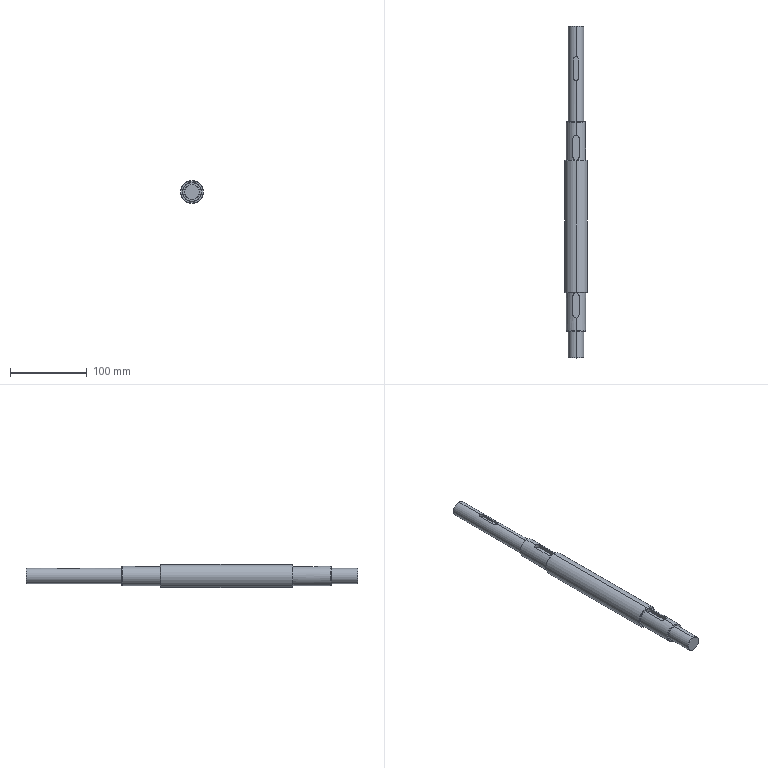Part | STEP file | LIELUN30_1-2 | 1 solid | 43 faces | box 30 x 432.6 x 30 mm | volume 218301 mm3 | cylinder 16 | plane 15 | cone 12 | commonest cylinder face diameters 8 x4 20 x4 25 x4 6 x2 30 x2
STEP:
#1=CARTESIAN_POINT('',(0.,85.5,15.));
#2=VERTEX_POINT('',#1);
#3=CARTESIAN_POINT('',(0.,85.5,-15.));
#4=VERTEX_POINT('',#3);
#5=CARTESIAN_POINT('',(0.,85.5,0.));
#6=DIRECTION('',(0.,1.,0.));
#7=DIRECTION('',(0.,0.,1.));
#8=AXIS2_PLACEMENT_3D('',#5,#6,#7);
#9=CIRCLE('',#8,15.);
#10=EDGE_CURVE('',#2,#4,#9,.T.);
#11=ORIENTED_EDGE('',*,*,#10,.T.);
#12=CARTESIAN_POINT('',(0.,257.1,-15.));
#13=VERTEX_POINT('',#12);
#14=CARTESIAN_POINT('',(0.,0.,-15.));
#15=DIRECTION('',(0.,1.,0.));
#16=VECTOR('',#15,1000.);
#17=LINE('',#14,#16);
#18=EDGE_CURVE('',#4,#13,#17,.T.);
#19=ORIENTED_EDGE('',*,*,#18,.T.);
#20=CARTESIAN_POINT('',(0.,257.1,15.));
#21=VERTEX_POINT('',#20);
#22=CARTESIAN_POINT('',(0.,257.1,0.));
#23=DIRECTION('',(0.,-1.,0.));
#24=DIRECTION('',(0.,0.,1.));
#25=AXIS2_PLACEMENT_3D('',#22,#23,#24);
#26=CIRCLE('',#25,15.);
#27=EDGE_CURVE('',#13,#21,#26,.T.);
#28=ORIENTED_EDGE('',*,*,#27,.T.);
#29=CARTESIAN_POINT('',(0.,0.,15.));
#30=DIRECTION('',(0.,1.,0.));
#31=VECTOR('',#30,1000.);
#32=LINE('',#29,#31);
#33=EDGE_CURVE('',#2,#21,#32,.T.);
#34=ORIENTED_EDGE('',*,*,#33,.F.);
#35=EDGE_LOOP('',(#11,#19,#28,#34));
#36=FACE_OUTER_BOUND('',#35,.T.);
#37=CARTESIAN_POINT('',(0.,0.,0.));
#38=DIRECTION('',(0.,1.,0.));
#39=DIRECTION('',(0.,0.,1.));
#40=AXIS2_PLACEMENT_3D('',#37,#38,#39);
#41=CYLINDRICAL_SURFACE('',#40,15.);
#42=ADVANCED_FACE('',(#36),#41,.T.);
#43=CARTESIAN_POINT('',(0.,257.6,-14.5));
#44=VERTEX_POINT('',#43);
#45=CARTESIAN_POINT('',(0.,257.6,14.5));
#46=VERTEX_POINT('',#45);
#47=CARTESIAN_POINT('',(0.,257.6,0.));
#48=DIRECTION('',(0.,-1.,0.));
#49=DIRECTION('',(0.,0.,-1.));
#50=AXIS2_PLACEMENT_3D('',#47,#48,#49);
#51=CIRCLE('',#50,14.5);
#52=EDGE_CURVE('',#44,#46,#51,.T.);
#53=ORIENTED_EDGE('',*,*,#52,.T.);
#54=CARTESIAN_POINT('',(0.,257.1,15.));
#55=DIRECTION('',(0.,-0.7071,0.7071));
#56=VECTOR('',#55,1000.);
#57=LINE('',#54,#56);
#58=EDGE_CURVE('',#46,#21,#57,.T.);
#59=ORIENTED_EDGE('',*,*,#58,.T.);
#60=ORIENTED_EDGE('',*,*,#27,.F.);
#61=CARTESIAN_POINT('',(0.,257.1,-15.));
#62=DIRECTION('',(0.,-0.7071,-0.7071));
#63=VECTOR('',#62,1000.);
#64=LINE('',#61,#63);
#65=EDGE_CURVE('',#44,#13,#64,.T.);
#66=ORIENTED_EDGE('',*,*,#65,.F.);
#67=EDGE_LOOP('',(#53,#59,#60,#66));
#68=FACE_OUTER_BOUND('',#67,.T.);
#69=CARTESIAN_POINT('',(0.,257.1,0.));
#70=DIRECTION('',(0.,-1.,0.));
#71=DIRECTION('',(0.,0.,-1.));
#72=AXIS2_PLACEMENT_3D('',#69,#70,#71);
#73=CONICAL_SURFACE('',#72,15.,0.7854);
#74=ADVANCED_FACE('',(#68),#73,.T.);
#75=CARTESIAN_POINT('',(0.,85.,14.5));
#76=VERTEX_POINT('',#75);
#77=CARTESIAN_POINT('',(0.,85.,-14.5));
#78=VERTEX_POINT('',#77);
#79=CARTESIAN_POINT('',(0.,85.,0.));
#80=DIRECTION('',(0.,1.,0.));
#81=DIRECTION('',(0.,0.,1.));
#82=AXIS2_PLACEMENT_3D('',#79,#80,#81);
#83=CIRCLE('',#82,14.5);
#84=EDGE_CURVE('',#76,#78,#83,.T.);
#85=ORIENTED_EDGE('',*,*,#84,.T.);
#86=CARTESIAN_POINT('',(0.,85.5,-15.));
#87=DIRECTION('',(0.,0.7071,-0.7071));
#88=VECTOR('',#87,1000.);
#89=LINE('',#86,#88);
#90=EDGE_CURVE('',#78,#4,#89,.T.);
#91=ORIENTED_EDGE('',*,*,#90,.T.);
#92=ORIENTED_EDGE('',*,*,#10,.F.);
#93=CARTESIAN_POINT('',(0.,85.5,15.));
#94=DIRECTION('',(0.,0.7071,0.7071));
#95=VECTOR('',#94,1000.);
#96=LINE('',#93,#95);
#97=EDGE_CURVE('',#76,#2,#96,.T.);
#98=ORIENTED_EDGE('',*,*,#97,.F.);
#99=EDGE_LOOP('',(#85,#91,#92,#98));
#100=FACE_OUTER_BOUND('',#99,.T.);
#101=CARTESIAN_POINT('',(0.,85.5,0.));
#102=DIRECTION('',(0.,1.,0.));
#103=DIRECTION('',(0.,0.,1.));
#104=AXIS2_PLACEMENT_3D('',#101,#102,#103);
#105=CONICAL_SURFACE('',#104,15.,0.7854);
#106=ADVANCED_FACE('',(#100),#105,.T.);
#107=CARTESIAN_POINT('',(0.,257.6,-12.5));
#108=VERTEX_POINT('',#107);
#109=CARTESIAN_POINT('',(0.,257.6,12.5));
#110=VERTEX_POINT('',#109);
#111=CARTESIAN_POINT('',(0.,257.6,0.));
#112=DIRECTION('',(0.,-1.,0.));
#113=DIRECTION('',(0.,0.,1.));
#114=AXIS2_PLACEMENT_3D('',#111,#112,#113);
#115=CIRCLE('',#114,12.5);
#116=EDGE_CURVE('',#108,#110,#115,.T.);
#117=ORIENTED_EDGE('',*,*,#116,.F.);
#118=CARTESIAN_POINT('',(0.,307.1,-12.5));
#119=VERTEX_POINT('',#118);
#120=CARTESIAN_POINT('',(0.,432.6,-12.5));
#121=DIRECTION('',(0.,1.,0.));
#122=VECTOR('',#121,1000.);
#123=LINE('',#120,#122);
#124=EDGE_CURVE('',#108,#119,#123,.T.);
#125=ORIENTED_EDGE('',*,*,#124,.T.);
#126=CARTESIAN_POINT('',(0.,307.1,12.5));
#127=VERTEX_POINT('',#126);
#128=CARTESIAN_POINT('',(0.,307.1,0.));
#129=DIRECTION('',(0.,-1.,0.));
#130=DIRECTION('',(0.,0.,1.));
#131=AXIS2_PLACEMENT_3D('',#128,#129,#130);
#132=CIRCLE('',#131,12.5);
#133=EDGE_CURVE('',#119,#127,#132,.T.);
#134=ORIENTED_EDGE('',*,*,#133,.T.);
#135=CARTESIAN_POINT('',(0.,290.6,12.5));
#136=VERTEX_POINT('',#135);
#137=CARTESIAN_POINT('',(0.,432.6,12.5));
#138=DIRECTION('',(0.,1.,0.));
#139=VECTOR('',#138,1000.);
#140=LINE('',#137,#139);
#141=EDGE_CURVE('',#136,#127,#140,.T.);
#142=ORIENTED_EDGE('',*,*,#141,.F.);
#143=CARTESIAN_POINT('',(4.,286.6,11.843));
#144=VERTEX_POINT('',#143);
#145=CARTESIAN_POINT('',(0.,290.6,12.5));
#146=CARTESIAN_POINT('',(0.266,290.6,12.5));
#147=CARTESIAN_POINT('',(0.5272,290.574,12.492));
#148=CARTESIAN_POINT('',(1.041,290.471,12.459));
#149=CARTESIAN_POINT('',(1.296,290.393,12.435));
#150=CARTESIAN_POINT('',(1.779,290.192,12.375));
#151=CARTESIAN_POINT('',(2.008,290.069,12.34));
#152=CARTESIAN_POINT('',(2.441,289.779,12.261));
#153=CARTESIAN_POINT('',(2.645,289.612,12.218));
#154=CARTESIAN_POINT('',(3.011,289.246,12.133));
#155=CARTESIAN_POINT('',(3.176,289.046,12.091));
#156=CARTESIAN_POINT('',(3.469,288.609,12.01));
#157=CARTESIAN_POINT('',(3.592,288.38,11.973));
#158=CARTESIAN_POINT('',(3.792,287.9,11.911));
#159=CARTESIAN_POINT('',(3.87,287.646,11.886));
#160=CARTESIAN_POINT('',(3.974,287.128,11.852));
#161=CARTESIAN_POINT('',(4.,286.866,11.843));
#162=CARTESIAN_POINT('',(4.,286.6,11.843));
#163=B_SPLINE_CURVE_WITH_KNOTS('',3,(#145,#146,#147,#148,#149,#150,#151,#152,#153,#154,#155,#156,#157,#158,#159,#160,#161,#162),.UNSPECIFIED.,.F.,.F.,(4,2,2,2,2,2,2,2,4),(0.00629,0.007077,0.007863,0.008649,0.009436,0.01022,0.01101,0.01179,0.01258),.UNSPECIFIED.);
#164=EDGE_CURVE('',#136,#144,#163,.T.);
#165=ORIENTED_EDGE('',*,*,#164,.T.);
#166=CARTESIAN_POINT('',(4.,261.6,11.843));
#167=VERTEX_POINT('',#166);
#168=CARTESIAN_POINT('',(4.,432.6,11.843));
#169=DIRECTION('',(0.,-1.,0.));
#170=VECTOR('',#169,1000.);
#171=LINE('',#168,#170);
#172=EDGE_CURVE('',#144,#167,#171,.T.);
#173=ORIENTED_EDGE('',*,*,#172,.T.);
#174=CARTESIAN_POINT('',(4.,261.6,11.843));
#175=CARTESIAN_POINT('',(4.,261.334,11.843));
#176=CARTESIAN_POINT('',(3.974,261.073,11.852));
#177=CARTESIAN_POINT('',(3.871,260.56,11.886));
#178=CARTESIAN_POINT('',(3.794,260.305,11.911));
#179=CARTESIAN_POINT('',(3.592,259.821,11.973));
#180=CARTESIAN_POINT('',(3.47,259.593,12.01));
#181=CARTESIAN_POINT('',(3.18,259.159,12.09));
#182=CARTESIAN_POINT('',(3.012,258.956,12.133));
#183=CARTESIAN_POINT('',(2.646,258.589,12.218));
#184=CARTESIAN_POINT('',(2.446,258.424,12.26));
#185=CARTESIAN_POINT('',(2.01,258.132,12.339));
#186=CARTESIAN_POINT('',(1.78,258.009,12.375));
#187=CARTESIAN_POINT('',(1.3,257.808,12.435));
#188=CARTESIAN_POINT('',(1.047,257.73,12.459));
#189=CARTESIAN_POINT('',(0.5285,257.626,12.492));
#190=CARTESIAN_POINT('',(0.266,257.6,12.5));
#191=CARTESIAN_POINT('',(0.,257.6,12.5));
#192=B_SPLINE_CURVE_WITH_KNOTS('',3,(#174,#175,#176,#177,#178,#179,#180,#181,#182,#183,#184,#185,#186,#187,#188,#189,#190,#191),.UNSPECIFIED.,.F.,.F.,(4,2,2,2,2,2,2,2,4),(0.,0.0007863,0.001573,0.002359,0.003145,0.003931,0.004718,0.005504,0.00629),.UNSPECIFIED.);
#193=EDGE_CURVE('',#167,#110,#192,.T.);
#194=ORIENTED_EDGE('',*,*,#193,.T.);
#195=EDGE_LOOP('',(#117,#125,#134,#142,#165,#173,#194));
#196=FACE_OUTER_BOUND('',#195,.T.);
#197=CARTESIAN_POINT('',(0.,432.6,0.));
#198=DIRECTION('',(0.,1.,0.));
#199=DIRECTION('',(0.,0.,1.));
#200=AXIS2_PLACEMENT_3D('',#197,#198,#199);
#201=CYLINDRICAL_SURFACE('',#200,12.5);
#202=ADVANCED_FACE('',(#196),#201,.T.);
#203=CARTESIAN_POINT('',(4.,56.,11.843));
#204=VERTEX_POINT('',#203);
#205=CARTESIAN_POINT('',(0.,52.,12.5));
#206=VERTEX_POINT('',#205);
#207=CARTESIAN_POINT('',(4.,56.,11.843));
#208=CARTESIAN_POINT('',(4.,55.734,11.843));
#209=CARTESIAN_POINT('',(3.974,55.473,11.852));
#210=CARTESIAN_POINT('',(3.871,54.96,11.886));
#211=CARTESIAN_POINT('',(3.794,54.705,11.911));
#212=CARTESIAN_POINT('',(3.592,54.221,11.973));
#213=CARTESIAN_POINT('',(3.47,53.993,12.01));
#214=CARTESIAN_POINT('',(3.18,53.559,12.09));
#215=CARTESIAN_POINT('',(3.012,53.356,12.133));
#216=CARTESIAN_POINT('',(2.646,52.989,12.218));
#217=CARTESIAN_POINT('',(2.446,52.824,12.26));
#218=CARTESIAN_POINT('',(2.01,52.532,12.339));
#219=CARTESIAN_POINT('',(1.78,52.409,12.375));
#220=CARTESIAN_POINT('',(1.3,52.208,12.435));
#221=CARTESIAN_POINT('',(1.047,52.13,12.459));
#222=CARTESIAN_POINT('',(0.5285,52.026,12.492));
#223=CARTESIAN_POINT('',(0.266,52.,12.5));
#224=CARTESIAN_POINT('',(0.,52.,12.5));
#225=B_SPLINE_CURVE_WITH_KNOTS('',3,(#207,#208,#209,#210,#211,#212,#213,#214,#215,#216,#217,#218,#219,#220,#221,#222,#223,#224),.UNSPECIFIED.,.F.,.F.,(4,2,2,2,2,2,2,2,4),(-0.00629,-0.005504,-0.004718,-0.003932,-0.003145,-0.002359,-0.001573,-0.0007863,0.),.UNSPECIFIED.);
#226=EDGE_CURVE('',#204,#206,#225,.T.);
#227=ORIENTED_EDGE('',*,*,#226,.T.);
#228=CARTESIAN_POINT('',(0.,35.5,12.5));
#229=VERTEX_POINT('',#228);
#230=CARTESIAN_POINT('',(0.,0.,12.5));
#231=DIRECTION('',(0.,-1.,0.));
#232=VECTOR('',#231,1000.);
#233=LINE('',#230,#232);
#234=EDGE_CURVE('',#206,#229,#233,.T.);
#235=ORIENTED_EDGE('',*,*,#234,.T.);
#236=CARTESIAN_POINT('',(12.5,35.5,0.));
#237=VERTEX_POINT('',#236);
#238=CARTESIAN_POINT('',(0.,35.5,0.));
#239=DIRECTION('',(0.,1.,0.));
#240=DIRECTION('',(0.,0.,-1.));
#241=AXIS2_PLACEMENT_3D('',#238,#239,#240);
#242=CIRCLE('',#241,12.5);
#243=EDGE_CURVE('',#229,#237,#242,.T.);
#244=ORIENTED_EDGE('',*,*,#243,.T.);
#245=CARTESIAN_POINT('',(0.,35.5,-12.5));
#246=VERTEX_POINT('',#245);
#247=CARTESIAN_POINT('',(0.,35.5,0.));
#248=DIRECTION('',(0.,1.,0.));
#249=DIRECTION('',(0.,0.,-1.));
#250=AXIS2_PLACEMENT_3D('',#247,#248,#249);
#251=CIRCLE('',#250,12.5);
#252=EDGE_CURVE('',#237,#246,#251,.T.);
#253=ORIENTED_EDGE('',*,*,#252,.T.);
#254=CARTESIAN_POINT('',(0.,85.,-12.5));
#255=VERTEX_POINT('',#254);
#256=CARTESIAN_POINT('',(0.,0.,-12.5));
#257=DIRECTION('',(0.,-1.,0.));
#258=VECTOR('',#257,1000.);
#259=LINE('',#256,#258);
#260=EDGE_CURVE('',#255,#246,#259,.T.);
#261=ORIENTED_EDGE('',*,*,#260,.F.);
#262=CARTESIAN_POINT('',(0.,85.,12.5));
#263=VERTEX_POINT('',#262);
#264=CARTESIAN_POINT('',(0.,85.,0.));
#265=DIRECTION('',(0.,1.,0.));
#266=DIRECTION('',(0.,0.,-1.));
#267=AXIS2_PLACEMENT_3D('',#264,#265,#266);
#268=CIRCLE('',#267,12.5);
#269=EDGE_CURVE('',#263,#255,#268,.T.);
#270=ORIENTED_EDGE('',*,*,#269,.F.);
#271=CARTESIAN_POINT('',(4.,81.,11.843));
#272=VERTEX_POINT('',#271);
#273=CARTESIAN_POINT('',(0.,85.,12.5));
#274=CARTESIAN_POINT('',(0.266,85.,12.5));
#275=CARTESIAN_POINT('',(0.5272,84.974,12.492));
#276=CARTESIAN_POINT('',(1.041,84.871,12.459));
#277=CARTESIAN_POINT('',(1.296,84.793,12.435));
#278=CARTESIAN_POINT('',(1.779,84.592,12.375));
#279=CARTESIAN_POINT('',(2.008,84.469,12.34));
#280=CARTESIAN_POINT('',(2.441,84.179,12.261));
#281=CARTESIAN_POINT('',(2.645,84.012,12.218));
#282=CARTESIAN_POINT('',(3.011,83.646,12.133));
#283=CARTESIAN_POINT('',(3.176,83.446,12.091));
#284=CARTESIAN_POINT('',(3.469,83.009,12.01));
#285=CARTESIAN_POINT('',(3.592,82.78,11.973));
#286=CARTESIAN_POINT('',(3.792,82.3,11.911));
#287=CARTESIAN_POINT('',(3.87,82.046,11.886));
#288=CARTESIAN_POINT('',(3.974,81.528,11.852));
#289=CARTESIAN_POINT('',(4.,81.266,11.843));
#290=CARTESIAN_POINT('',(4.,81.,11.843));
#291=B_SPLINE_CURVE_WITH_KNOTS('',3,(#273,#274,#275,#276,#277,#278,#279,#280,#281,#282,#283,#284,#285,#286,#287,#288,#289,#290),.UNSPECIFIED.,.F.,.F.,(4,2,2,2,2,2,2,2,4),(0.,0.0007863,0.001573,0.002359,0.003145,0.003932,0.004718,0.005504,0.00629),.UNSPECIFIED.);
#292=EDGE_CURVE('',#263,#272,#291,.T.);
#293=ORIENTED_EDGE('',*,*,#292,.T.);
#294=CARTESIAN_POINT('',(4.,0.,11.843));
#295=DIRECTION('',(0.,-1.,0.));
#296=VECTOR('',#295,1000.);
#297=LINE('',#294,#296);
#298=EDGE_CURVE('',#272,#204,#297,.T.);
#299=ORIENTED_EDGE('',*,*,#298,.T.);
#300=EDGE_LOOP('',(#227,#235,#244,#253,#261,#270,#293,#299));
#301=FACE_OUTER_BOUND('',#300,.T.);
#302=CARTESIAN_POINT('',(0.,0.,0.));
#303=DIRECTION('',(0.,-1.,0.));
#304=DIRECTION('',(0.,0.,-1.));
#305=AXIS2_PLACEMENT_3D('',#302,#303,#304);
#306=CYLINDRICAL_SURFACE('',#305,12.5);
#307=ADVANCED_FACE('',(#301),#306,.T.);
#308=CARTESIAN_POINT('',(0.,307.6,-12.));
#309=VERTEX_POINT('',#308);
#310=CARTESIAN_POINT('',(0.,307.6,12.));
#311=VERTEX_POINT('',#310);
#312=CARTESIAN_POINT('',(0.,307.6,0.));
#313=DIRECTION('',(0.,-1.,0.));
#314=DIRECTION('',(0.,0.,-1.));
#315=AXIS2_PLACEMENT_3D('',#312,#313,#314);
#316=CIRCLE('',#315,12.);
#317=EDGE_CURVE('',#309,#311,#316,.T.);
#318=ORIENTED_EDGE('',*,*,#317,.T.);
#319=CARTESIAN_POINT('',(0.,307.1,12.5));
#320=DIRECTION('',(0.,-0.7071,0.7071));
#321=VECTOR('',#320,1000.);
#322=LINE('',#319,#321);
#323=EDGE_CURVE('',#311,#127,#322,.T.);
#324=ORIENTED_EDGE('',*,*,#323,.T.);
#325=ORIENTED_EDGE('',*,*,#133,.F.);
#326=CARTESIAN_POINT('',(0.,307.1,-12.5));
#327=DIRECTION('',(0.,-0.7071,-0.7071));
#328=VECTOR('',#327,1000.);
#329=LINE('',#326,#328);
#330=EDGE_CURVE('',#309,#119,#329,.T.);
#331=ORIENTED_EDGE('',*,*,#330,.F.);
#332=EDGE_LOOP('',(#318,#324,#325,#331));
#333=FACE_OUTER_BOUND('',#332,.T.);
#334=CARTESIAN_POINT('',(0.,307.1,0.));
#335=DIRECTION('',(0.,-1.,0.));
#336=DIRECTION('',(0.,0.,-1.));
#337=AXIS2_PLACEMENT_3D('',#334,#335,#336);
#338=CONICAL_SURFACE('',#337,12.5,0.7854);
#339=ADVANCED_FACE('',(#333),#338,.T.);
#340=CARTESIAN_POINT('',(-12.,35.,0.));
#341=VERTEX_POINT('',#340);
#342=CARTESIAN_POINT('',(12.,35.,0.));
#343=VERTEX_POINT('',#342);
#344=CARTESIAN_POINT('',(0.,35.,0.));
#345=DIRECTION('',(0.,1.,0.));
#346=DIRECTION('',(-1.,0.,0.));
#347=AXIS2_PLACEMENT_3D('',#344,#345,#346);
#348=CIRCLE('',#347,12.);
#349=EDGE_CURVE('',#341,#343,#348,.T.);
#350=ORIENTED_EDGE('',*,*,#349,.T.);
#351=CARTESIAN_POINT('',(12.5,35.5,0.));
#352=DIRECTION('',(0.7071,0.7071,0.));
#353=VECTOR('',#352,1000.);
#354=LINE('',#351,#353);
#355=EDGE_CURVE('',#343,#237,#354,.T.);
#356=ORIENTED_EDGE('',*,*,#355,.T.);
#357=ORIENTED_EDGE('',*,*,#243,.F.);
#358=CARTESIAN_POINT('',(-12.5,35.5,0.));
#359=VERTEX_POINT('',#358);
#360=CARTESIAN_POINT('',(0.,35.5,0.));
#361=DIRECTION('',(0.,1.,0.));
#362=DIRECTION('',(0.,0.,-1.));
#363=AXIS2_PLACEMENT_3D('',#360,#361,#362);
#364=CIRCLE('',#363,12.5);
#365=EDGE_CURVE('',#359,#229,#364,.T.);
#366=ORIENTED_EDGE('',*,*,#365,.F.);
#367=CARTESIAN_POINT('',(-12.5,35.5,0.));
#368=DIRECTION('',(-0.7071,0.7071,0.));
#369=VECTOR('',#368,1000.);
#370=LINE('',#367,#369);
#371=EDGE_CURVE('',#341,#359,#370,.T.);
#372=ORIENTED_EDGE('',*,*,#371,.F.);
#373=EDGE_LOOP('',(#350,#356,#357,#366,#372));
#374=FACE_OUTER_BOUND('',#373,.T.);
#375=CARTESIAN_POINT('',(0.,35.5,0.));
#376=DIRECTION('',(0.,1.,0.));
#377=DIRECTION('',(-1.,0.,0.));
#378=AXIS2_PLACEMENT_3D('',#375,#376,#377);
#379=CONICAL_SURFACE('',#378,12.5,0.7854);
#380=ADVANCED_FACE('',(#374),#379,.T.);
#381=CARTESIAN_POINT('',(0.,307.6,-10.));
#382=VERTEX_POINT('',#381);
#383=CARTESIAN_POINT('',(0.,307.6,10.));
#384=VERTEX_POINT('',#383);
#385=CARTESIAN_POINT('',(0.,307.6,0.));
#386=DIRECTION('',(0.,-1.,0.));
#387=DIRECTION('',(0.,0.,1.));
#388=AXIS2_PLACEMENT_3D('',#385,#386,#387);
#389=CIRCLE('',#388,10.);
#390=EDGE_CURVE('',#382,#384,#389,.T.);
#391=ORIENTED_EDGE('',*,*,#390,.F.);
#392=CARTESIAN_POINT('',(0.,432.1,-10.));
#393=VERTEX_POINT('',#392);
#394=CARTESIAN_POINT('',(0.,432.6,-10.));
#395=DIRECTION('',(0.,1.,0.));
#396=VECTOR('',#395,1000.);
#397=LINE('',#394,#396);
#398=EDGE_CURVE('',#382,#393,#397,.T.);
#399=ORIENTED_EDGE('',*,*,#398,.T.);
#400=CARTESIAN_POINT('',(0.,432.1,10.));
#401=VERTEX_POINT('',#400);
#402=CARTESIAN_POINT('',(0.,432.1,0.));
#403=DIRECTION('',(0.,-1.,0.));
#404=DIRECTION('',(0.,0.,1.));
#405=AXIS2_PLACEMENT_3D('',#402,#403,#404);
#406=CIRCLE('',#405,10.);
#407=EDGE_CURVE('',#393,#401,#406,.T.);
#408=ORIENTED_EDGE('',*,*,#407,.T.);
#409=CARTESIAN_POINT('',(0.,392.6,10.));
#410=VERTEX_POINT('',#409);
#411=CARTESIAN_POINT('',(0.,432.6,10.));
#412=DIRECTION('',(0.,1.,0.));
#413=VECTOR('',#412,1000.);
#414=LINE('',#411,#413);
#415=EDGE_CURVE('',#410,#401,#414,.T.);
#416=ORIENTED_EDGE('',*,*,#415,.F.);
#417=CARTESIAN_POINT('',(3.,389.6,9.539));
#418=VERTEX_POINT('',#417);
#419=CARTESIAN_POINT('',(0.,392.6,10.));
#420=CARTESIAN_POINT('',(0.1993,392.6,10.));
#421=CARTESIAN_POINT('',(0.3951,392.58,9.994));
#422=CARTESIAN_POINT('',(0.7799,392.503,9.971));
#423=CARTESIAN_POINT('',(0.971,392.445,9.954));
#424=CARTESIAN_POINT('',(1.334,392.294,9.912));
#425=CARTESIAN_POINT('',(1.505,392.202,9.887));
#426=CARTESIAN_POINT('',(1.831,391.985,9.832));
#427=CARTESIAN_POINT('',(1.984,391.859,9.802));
#428=CARTESIAN_POINT('',(2.396,391.447,9.713));
#429=CARTESIAN_POINT('',(2.619,391.114,9.652));
#430=CARTESIAN_POINT('',(2.844,390.574,9.587));
#431=CARTESIAN_POINT('',(2.902,390.384,9.57));
#432=CARTESIAN_POINT('',(2.98,389.996,9.546));
#433=CARTESIAN_POINT('',(3.,389.799,9.539));
#434=CARTESIAN_POINT('',(3.,389.6,9.539));
#435=B_SPLINE_CURVE_WITH_KNOTS('',3,(#419,#420,#421,#422,#423,#424,#425,#426,#427,#428,#429,#430,#431,#432,#433,#434),.UNSPECIFIED.,.F.,.F.,(4,2,2,2,2,2,2,4),(0.004714,0.005303,0.005892,0.006481,0.007071,0.008249,0.008838,0.009428),.UNSPECIFIED.);
#436=EDGE_CURVE('',#410,#418,#435,.T.);
#437=ORIENTED_EDGE('',*,*,#436,.T.);
#438=CARTESIAN_POINT('',(3.,364.6,9.539));
#439=VERTEX_POINT('',#438);
#440=CARTESIAN_POINT('',(3.,432.6,9.539));
#441=DIRECTION('',(0.,-1.,0.));
#442=VECTOR('',#441,1000.);
#443=LINE('',#440,#442);
#444=EDGE_CURVE('',#418,#439,#443,.T.);
#445=ORIENTED_EDGE('',*,*,#444,.T.);
#446=CARTESIAN_POINT('',(0.,361.6,10.));
#447=VERTEX_POINT('',#446);
#448=CARTESIAN_POINT('',(3.,364.6,9.539));
#449=CARTESIAN_POINT('',(3.,364.401,9.539));
#450=CARTESIAN_POINT('',(2.98,364.205,9.546));
#451=CARTESIAN_POINT('',(2.904,363.82,9.569));
#452=CARTESIAN_POINT('',(2.845,363.629,9.587));
#453=CARTESIAN_POINT('',(2.695,363.267,9.63));
#454=CARTESIAN_POINT('',(2.602,363.095,9.656));
#455=CARTESIAN_POINT('',(2.385,362.77,9.712));
#456=CARTESIAN_POINT('',(2.259,362.617,9.742));
#457=CARTESIAN_POINT('',(1.847,362.204,9.832));
#458=CARTESIAN_POINT('',(1.515,361.981,9.891));
#459=CARTESIAN_POINT('',(0.9743,361.756,9.954));
#460=CARTESIAN_POINT('',(0.7845,361.698,9.971));
#461=CARTESIAN_POINT('',(0.3961,361.62,9.994));
#462=CARTESIAN_POINT('',(0.1993,361.6,10.));
#463=CARTESIAN_POINT('',(0.,361.6,10.));
#464=B_SPLINE_CURVE_WITH_KNOTS('',3,(#448,#449,#450,#451,#452,#453,#454,#455,#456,#457,#458,#459,#460,#461,#462,#463),.UNSPECIFIED.,.F.,.F.,(4,2,2,2,2,2,2,4),(-0.004714,-0.004125,-0.003535,-0.002946,-0.002357,-0.001178,-0.0005892,0.),.UNSPECIFIED.);
#465=EDGE_CURVE('',#439,#447,#464,.T.);
#466=ORIENTED_EDGE('',*,*,#465,.T.);
#467=CARTESIAN_POINT('',(0.,432.6,10.));
#468=DIRECTION('',(0.,1.,0.));
#469=VECTOR('',#468,1000.);
#470=LINE('',#467,#469);
#471=EDGE_CURVE('',#384,#447,#470,.T.);
#472=ORIENTED_EDGE('',*,*,#471,.F.);
#473=EDGE_LOOP('',(#391,#399,#408,#416,#437,#445,#466,#472));
#474=FACE_OUTER_BOUND('',#473,.T.);
#475=CARTESIAN_POINT('',(0.,432.6,0.));
#476=DIRECTION('',(0.,1.,0.));
#477=DIRECTION('',(0.,0.,1.));
#478=AXIS2_PLACEMENT_3D('',#475,#476,#477);
#479=CYLINDRICAL_SURFACE('',#478,10.);
#480=ADVANCED_FACE('',(#474),#479,.T.);
#481=CARTESIAN_POINT('',(0.,35.,10.));
#482=VERTEX_POINT('',#481);
#483=CARTESIAN_POINT('',(0.,35.,-10.));
#484=VERTEX_POINT('',#483);
#485=CARTESIAN_POINT('',(0.,35.,0.));
#486=DIRECTION('',(0.,1.,0.));
#487=DIRECTION('',(0.,0.,-1.));
#488=AXIS2_PLACEMENT_3D('',#485,#486,#487);
#489=CIRCLE('',#488,10.);
#490=EDGE_CURVE('',#482,#484,#489,.T.);
#491=ORIENTED_EDGE('',*,*,#490,.F.);
#492=CARTESIAN_POINT('',(0.,0.5,10.));
#493=VERTEX_POINT('',#492);
#494=CARTESIAN_POINT('',(0.,0.,10.));
#495=DIRECTION('',(0.,-1.,0.));
#496=VECTOR('',#495,1000.);
#497=LINE('',#494,#496);
#498=EDGE_CURVE('',#482,#493,#497,.T.);
#499=ORIENTED_EDGE('',*,*,#498,.T.);
#500=CARTESIAN_POINT('',(0.,0.5,-10.));
#501=VERTEX_POINT('',#500);
#502=CARTESIAN_POINT('',(0.,0.5,0.));
#503=DIRECTION('',(0.,1.,0.));
#504=DIRECTION('',(0.,0.,-1.));
#505=AXIS2_PLACEMENT_3D('',#502,#503,#504);
#506=CIRCLE('',#505,10.);
#507=EDGE_CURVE('',#493,#501,#506,.T.);
#508=ORIENTED_EDGE('',*,*,#507,.T.);
#509=CARTESIAN_POINT('',(0.,0.,-10.));
#510=DIRECTION('',(0.,-1.,0.));
#511=VECTOR('',#510,1000.);
#512=LINE('',#509,#511);
#513=EDGE_CURVE('',#484,#501,#512,.T.);
#514=ORIENTED_EDGE('',*,*,#513,.F.);
#515=EDGE_LOOP('',(#491,#499,#508,#514));
#516=FACE_OUTER_BOUND('',#515,.T.);
#517=CARTESIAN_POINT('',(0.,0.,0.));
#518=DIRECTION('',(0.,-1.,0.));
#519=DIRECTION('',(0.,0.,-1.));
#520=AXIS2_PLACEMENT_3D('',#517,#518,#519);
#521=CYLINDRICAL_SURFACE('',#520,10.);
#522=ADVANCED_FACE('',(#516),#521,.T.);
#523=CARTESIAN_POINT('',(0.,432.6,-9.5));
#524=VERTEX_POINT('',#523);
#525=CARTESIAN_POINT('',(0.,432.6,9.5));
#526=VERTEX_POINT('',#525);
#527=CARTESIAN_POINT('',(0.,432.6,0.));
#528=DIRECTION('',(0.,-1.,0.));
#529=DIRECTION('',(0.,0.,-1.));
#530=AXIS2_PLACEMENT_3D('',#527,#528,#529);
#531=CIRCLE('',#530,9.5);
#532=EDGE_CURVE('',#524,#526,#531,.T.);
#533=ORIENTED_EDGE('',*,*,#532,.T.);
#534=CARTESIAN_POINT('',(0.,432.1,10.));
#535=DIRECTION('',(0.,-0.7071,0.7071));
#536=VECTOR('',#535,1000.);
#537=LINE('',#534,#536);
#538=EDGE_CURVE('',#526,#401,#537,.T.);
#539=ORIENTED_EDGE('',*,*,#538,.T.);
#540=ORIENTED_EDGE('',*,*,#407,.F.);
#541=CARTESIAN_POINT('',(0.,432.1,-10.));
#542=DIRECTION('',(0.,-0.7071,-0.7071));
#543=VECTOR('',#542,1000.);
#544=LINE('',#541,#543);
#545=EDGE_CURVE('',#524,#393,#544,.T.);
#546=ORIENTED_EDGE('',*,*,#545,.F.);
#547=EDGE_LOOP('',(#533,#539,#540,#546));
#548=FACE_OUTER_BOUND('',#547,.T.);
#549=CARTESIAN_POINT('',(0.,432.1,0.));
#550=DIRECTION('',(0.,-1.,0.));
#551=DIRECTION('',(0.,0.,-1.));
#552=AXIS2_PLACEMENT_3D('',#549,#550,#551);
#553=CONICAL_SURFACE('',#552,10.,0.7854);
#554=ADVANCED_FACE('',(#548),#553,.T.);
#555=CARTESIAN_POINT('',(0.,0.,9.5));
#556=VERTEX_POINT('',#555);
#557=CARTESIAN_POINT('',(0.,0.,-9.5));
#558=VERTEX_POINT('',#557);
#559=CARTESIAN_POINT('',(0.,0.,0.));
#560=DIRECTION('',(0.,1.,0.));
#561=DIRECTION('',(0.,0.,1.));
#562=AXIS2_PLACEMENT_3D('',#559,#560,#561);
#563=CIRCLE('',#562,9.5);
#564=EDGE_CURVE('',#556,#558,#563,.T.);
#565=ORIENTED_EDGE('',*,*,#564,.T.);
#566=CARTESIAN_POINT('',(0.,0.5,-10.));
#567=DIRECTION('',(0.,0.7071,-0.7071));
#568=VECTOR('',#567,1000.);
#569=LINE('',#566,#568);
#570=EDGE_CURVE('',#558,#501,#569,.T.);
#571=ORIENTED_EDGE('',*,*,#570,.T.);
#572=ORIENTED_EDGE('',*,*,#507,.F.);
#573=CARTESIAN_POINT('',(0.,0.5,10.));
#574=DIRECTION('',(0.,0.7071,0.7071));
#575=VECTOR('',#574,1000.);
#576=LINE('',#573,#575);
#577=EDGE_CURVE('',#556,#493,#576,.T.);
#578=ORIENTED_EDGE('',*,*,#577,.F.);
#579=EDGE_LOOP('',(#565,#571,#572,#578));
#580=FACE_OUTER_BOUND('',#579,.T.);
#581=CARTESIAN_POINT('',(0.,0.5,0.));
#582=DIRECTION('',(0.,1.,0.));
#583=DIRECTION('',(0.,0.,1.));
#584=AXIS2_PLACEMENT_3D('',#581,#582,#583);
#585=CONICAL_SURFACE('',#584,10.,0.7854);
#586=ADVANCED_FACE('',(#580),#585,.T.);
#587=ORIENTED_EDGE('',*,*,#18,.F.);
#588=CARTESIAN_POINT('',(0.,85.5,0.));
#589=DIRECTION('',(0.,1.,0.));
#590=DIRECTION('',(0.,0.,1.));
#591=AXIS2_PLACEMENT_3D('',#588,#589,#590);
#592=CIRCLE('',#591,15.);
#593=EDGE_CURVE('',#4,#2,#592,.T.);
#594=ORIENTED_EDGE('',*,*,#593,.T.);
#595=ORIENTED_EDGE('',*,*,#33,.T.);
#596=CARTESIAN_POINT('',(0.,257.1,0.));
#597=DIRECTION('',(0.,-1.,0.));
#598=DIRECTION('',(0.,0.,1.));
#599=AXIS2_PLACEMENT_3D('',#596,#597,#598);
#600=CIRCLE('',#599,15.);
#601=EDGE_CURVE('',#21,#13,#600,.T.);
#602=ORIENTED_EDGE('',*,*,#601,.T.);
#603=EDGE_LOOP('',(#587,#594,#595,#602));
#604=FACE_OUTER_BOUND('',#603,.T.);
#605=CARTESIAN_POINT('',(0.,0.,0.));
#606=DIRECTION('',(0.,1.,0.));
#607=DIRECTION('',(0.,0.,1.));
#608=AXIS2_PLACEMENT_3D('',#605,#606,#607);
#609=CYLINDRICAL_SURFACE('',#608,15.);
#610=ADVANCED_FACE('',(#604),#609,.T.);
#611=ORIENTED_EDGE('',*,*,#58,.F.);
#612=CARTESIAN_POINT('',(0.,257.6,0.));
#613=DIRECTION('',(0.,-1.,0.));
#614=DIRECTION('',(0.,0.,-1.));
#615=AXIS2_PLACEMENT_3D('',#612,#613,#614);
#616=CIRCLE('',#615,14.5);
#617=EDGE_CURVE('',#46,#44,#616,.T.);
#618=ORIENTED_EDGE('',*,*,#617,.T.);
#619=ORIENTED_EDGE('',*,*,#65,.T.);
#620=ORIENTED_EDGE('',*,*,#601,.F.);
#621=EDGE_LOOP('',(#611,#618,#619,#620));
#622=FACE_OUTER_BOUND('',#621,.T.);
#623=CARTESIAN_POINT('',(0.,257.1,0.));
#624=DIRECTION('',(0.,-1.,0.));
#625=DIRECTION('',(0.,0.,-1.));
#626=AXIS2_PLACEMENT_3D('',#623,#624,#625);
#627=CONICAL_SURFACE('',#626,15.,0.7854);
#628=ADVANCED_FACE('',(#622),#627,.T.);
#629=ORIENTED_EDGE('',*,*,#90,.F.);
#630=CARTESIAN_POINT('',(0.,85.,0.));
#631=DIRECTION('',(0.,1.,0.));
#632=DIRECTION('',(0.,0.,1.));
#633=AXIS2_PLACEMENT_3D('',#630,#631,#632);
#634=CIRCLE('',#633,14.5);
#635=EDGE_CURVE('',#78,#76,#634,.T.);
#636=ORIENTED_EDGE('',*,*,#635,.T.);
#637=ORIENTED_EDGE('',*,*,#97,.T.);
#638=ORIENTED_EDGE('',*,*,#593,.F.);
#639=EDGE_LOOP('',(#629,#636,#637,#638));
#640=FACE_OUTER_BOUND('',#639,.T.);
#641=CARTESIAN_POINT('',(0.,85.5,0.));
#642=DIRECTION('',(0.,1.,0.));
#643=DIRECTION('',(0.,0.,1.));
#644=AXIS2_PLACEMENT_3D('',#641,#642,#643);
#645=CONICAL_SURFACE('',#644,15.,0.7854);
#646=ADVANCED_FACE('',(#640),#645,.T.);
#647=CARTESIAN_POINT('',(0.,257.6,0.));
#648=DIRECTION('',(0.,-1.,0.));
#649=DIRECTION('',(0.,0.,1.));
#650=AXIS2_PLACEMENT_3D('',#647,#648,#649);
#651=CIRCLE('',#650,12.5);
#652=EDGE_CURVE('',#110,#108,#651,.T.);
#653=ORIENTED_EDGE('',*,*,#652,.T.);
#654=ORIENTED_EDGE('',*,*,#116,.T.);
#655=EDGE_LOOP('',(#653,#654));
#656=FACE_BOUND('',#655,.T.);
#657=ORIENTED_EDGE('',*,*,#52,.F.);
#658=ORIENTED_EDGE('',*,*,#617,.F.);
#659=EDGE_LOOP('',(#657,#658));
#660=FACE_OUTER_BOUND('',#659,.T.);
#661=CARTESIAN_POINT('',(0.,257.6,0.));
#662=DIRECTION('',(0.,1.,0.));
#663=DIRECTION('',(0.,0.,1.));
#664=AXIS2_PLACEMENT_3D('',#661,#662,#663);
#665=PLANE('',#664);
#666=ADVANCED_FACE('',(#656,#660),#665,.T.);
#667=ORIENTED_EDGE('',*,*,#269,.T.);
#668=CARTESIAN_POINT('',(0.,85.,0.));
#669=DIRECTION('',(0.,1.,0.));
#670=DIRECTION('',(0.,0.,-1.));
#671=AXIS2_PLACEMENT_3D('',#668,#669,#670);
#672=CIRCLE('',#671,12.5);
#673=EDGE_CURVE('',#255,#263,#672,.T.);
#674=ORIENTED_EDGE('',*,*,#673,.T.);
#675=EDGE_LOOP('',(#667,#674));
#676=FACE_BOUND('',#675,.T.);
#677=ORIENTED_EDGE('',*,*,#84,.F.);
#678=ORIENTED_EDGE('',*,*,#635,.F.);
#679=EDGE_LOOP('',(#677,#678));
#680=FACE_OUTER_BOUND('',#679,.T.);
#681=CARTESIAN_POINT('',(0.,85.,0.));
#682=DIRECTION('',(0.,-1.,0.));
#683=DIRECTION('',(0.,0.,-1.));
#684=AXIS2_PLACEMENT_3D('',#681,#682,#683);
#685=PLANE('',#684);
#686=ADVANCED_FACE('',(#676,#680),#685,.T.);
#687=ORIENTED_EDGE('',*,*,#124,.F.);
#688=ORIENTED_EDGE('',*,*,#652,.F.);
#689=CARTESIAN_POINT('',(-4.,261.6,11.843));
#690=VERTEX_POINT('',#689);
#691=CARTESIAN_POINT('',(0.,257.6,12.5));
#692=CARTESIAN_POINT('',(-0.266,257.6,12.5));
#693=CARTESIAN_POINT('',(-0.5272,257.626,12.492));
#694=CARTESIAN_POINT('',(-1.041,257.729,12.459));
#695=CARTESIAN_POINT('',(-1.296,257.807,12.435));
#696=CARTESIAN_POINT('',(-1.779,258.008,12.375));
#697=CARTESIAN_POINT('',(-2.008,258.131,12.34));
#698=CARTESIAN_POINT('',(-2.441,258.421,12.261));
#699=CARTESIAN_POINT('',(-2.645,258.588,12.218));
#700=CARTESIAN_POINT('',(-3.011,258.954,12.133));
#701=CARTESIAN_POINT('',(-3.176,259.154,12.091));
#702=CARTESIAN_POINT('',(-3.469,259.591,12.01));
#703=CARTESIAN_POINT('',(-3.592,259.82,11.973));
#704=CARTESIAN_POINT('',(-3.792,260.3,11.911));
#705=CARTESIAN_POINT('',(-3.87,260.554,11.886));
#706=CARTESIAN_POINT('',(-3.974,261.072,11.852));
#707=CARTESIAN_POINT('',(-4.,261.334,11.843));
#708=CARTESIAN_POINT('',(-4.,261.6,11.843));
#709=B_SPLINE_CURVE_WITH_KNOTS('',3,(#691,#692,#693,#694,#695,#696,#697,#698,#699,#700,#701,#702,#703,#704,#705,#706,#707,#708),.UNSPECIFIED.,.F.,.F.,(4,2,2,2,2,2,2,2,4),(0.,0.0007863,0.001573,0.002359,0.003145,0.003932,0.004718,0.005504,0.00629),.UNSPECIFIED.);
#710=EDGE_CURVE('',#110,#690,#709,.T.);
#711=ORIENTED_EDGE('',*,*,#710,.T.);
#712=CARTESIAN_POINT('',(-4.,286.6,11.843));
#713=VERTEX_POINT('',#712);
#714=CARTESIAN_POINT('',(-4.,432.6,11.843));
#715=DIRECTION('',(0.,1.,0.));
#716=VECTOR('',#715,1000.);
#717=LINE('',#714,#716);
#718=EDGE_CURVE('',#690,#713,#717,.T.);
#719=ORIENTED_EDGE('',*,*,#718,.T.);
#720=CARTESIAN_POINT('',(-4.,286.6,11.843));
#721=CARTESIAN_POINT('',(-4.,286.866,11.843));
#722=CARTESIAN_POINT('',(-3.974,287.127,11.852));
#723=CARTESIAN_POINT('',(-3.871,287.64,11.886));
#724=CARTESIAN_POINT('',(-3.794,287.895,11.911));
#725=CARTESIAN_POINT('',(-3.592,288.379,11.973));
#726=CARTESIAN_POINT('',(-3.47,288.607,12.01));
#727=CARTESIAN_POINT('',(-3.18,289.041,12.09));
#728=CARTESIAN_POINT('',(-3.012,289.244,12.133));
#729=CARTESIAN_POINT('',(-2.646,289.611,12.218));
#730=CARTESIAN_POINT('',(-2.446,289.776,12.26));
#731=CARTESIAN_POINT('',(-2.01,290.068,12.339));
#732=CARTESIAN_POINT('',(-1.78,290.191,12.375));
#733=CARTESIAN_POINT('',(-1.3,290.392,12.435));
#734=CARTESIAN_POINT('',(-1.047,290.47,12.459));
#735=CARTESIAN_POINT('',(-0.5285,290.574,12.492));
#736=CARTESIAN_POINT('',(-0.266,290.6,12.5));
#737=CARTESIAN_POINT('',(0.,290.6,12.5));
#738=B_SPLINE_CURVE_WITH_KNOTS('',3,(#720,#721,#722,#723,#724,#725,#726,#727,#728,#729,#730,#731,#732,#733,#734,#735,#736,#737),.UNSPECIFIED.,.F.,.F.,(4,2,2,2,2,2,2,2,4),(0.,0.0007863,0.001573,0.002359,0.003145,0.003931,0.004718,0.005504,0.00629),.UNSPECIFIED.);
#739=EDGE_CURVE('',#713,#136,#738,.T.);
#740=ORIENTED_EDGE('',*,*,#739,.T.);
#741=ORIENTED_EDGE('',*,*,#141,.T.);
#742=CARTESIAN_POINT('',(0.,307.1,0.));
#743=DIRECTION('',(0.,-1.,0.));
#744=DIRECTION('',(0.,0.,1.));
#745=AXIS2_PLACEMENT_3D('',#742,#743,#744);
#746=CIRCLE('',#745,12.5);
#747=EDGE_CURVE('',#127,#119,#746,.T.);
#748=ORIENTED_EDGE('',*,*,#747,.T.);
#749=EDGE_LOOP('',(#687,#688,#711,#719,#740,#741,#748));
#750=FACE_OUTER_BOUND('',#749,.T.);
#751=CARTESIAN_POINT('',(0.,432.6,0.));
#752=DIRECTION('',(0.,1.,0.));
#753=DIRECTION('',(0.,0.,1.));
#754=AXIS2_PLACEMENT_3D('',#751,#752,#753);
#755=CYLINDRICAL_SURFACE('',#754,12.5);
#756=ADVANCED_FACE('',(#750),#755,.T.);
#757=ORIENTED_EDGE('',*,*,#234,.F.);
#758=CARTESIAN_POINT('',(-4.,56.,11.843));
#759=VERTEX_POINT('',#758);
#760=CARTESIAN_POINT('',(0.,52.,12.5));
#761=CARTESIAN_POINT('',(-0.266,52.,12.5));
#762=CARTESIAN_POINT('',(-0.5272,52.026,12.492));
#763=CARTESIAN_POINT('',(-1.041,52.129,12.459));
#764=CARTESIAN_POINT('',(-1.296,52.207,12.435));
#765=CARTESIAN_POINT('',(-1.779,52.408,12.375));
#766=CARTESIAN_POINT('',(-2.008,52.531,12.34));
#767=CARTESIAN_POINT('',(-2.441,52.821,12.261));
#768=CARTESIAN_POINT('',(-2.645,52.988,12.218));
#769=CARTESIAN_POINT('',(-3.011,53.354,12.133));
#770=CARTESIAN_POINT('',(-3.176,53.554,12.091));
#771=CARTESIAN_POINT('',(-3.469,53.991,12.01));
#772=CARTESIAN_POINT('',(-3.592,54.22,11.973));
#773=CARTESIAN_POINT('',(-3.792,54.7,11.911));
#774=CARTESIAN_POINT('',(-3.87,54.954,11.886));
#775=CARTESIAN_POINT('',(-3.974,55.472,11.852));
#776=CARTESIAN_POINT('',(-4.,55.734,11.843));
#777=CARTESIAN_POINT('',(-4.,56.,11.843));
#778=B_SPLINE_CURVE_WITH_KNOTS('',3,(#760,#761,#762,#763,#764,#765,#766,#767,#768,#769,#770,#771,#772,#773,#774,#775,#776,#777),.UNSPECIFIED.,.F.,.F.,(4,2,2,2,2,2,2,2,4),(0.,0.0007863,0.001573,0.002359,0.003145,0.003932,0.004718,0.005504,0.00629),.UNSPECIFIED.);
#779=EDGE_CURVE('',#206,#759,#778,.T.);
#780=ORIENTED_EDGE('',*,*,#779,.T.);
#781=CARTESIAN_POINT('',(-4.,81.,11.843));
#782=VERTEX_POINT('',#781);
#783=CARTESIAN_POINT('',(-4.,0.,11.843));
#784=DIRECTION('',(0.,1.,0.));
#785=VECTOR('',#784,1000.);
#786=LINE('',#783,#785);
#787=EDGE_CURVE('',#759,#782,#786,.T.);
#788=ORIENTED_EDGE('',*,*,#787,.T.);
#789=CARTESIAN_POINT('',(-4.,81.,11.843));
#790=CARTESIAN_POINT('',(-4.,81.266,11.843));
#791=CARTESIAN_POINT('',(-3.974,81.527,11.852));
#792=CARTESIAN_POINT('',(-3.871,82.04,11.886));
#793=CARTESIAN_POINT('',(-3.794,82.295,11.911));
#794=CARTESIAN_POINT('',(-3.592,82.779,11.973));
#795=CARTESIAN_POINT('',(-3.47,83.007,12.01));
#796=CARTESIAN_POINT('',(-3.18,83.441,12.09));
#797=CARTESIAN_POINT('',(-3.012,83.644,12.133));
#798=CARTESIAN_POINT('',(-2.646,84.011,12.218));
#799=CARTESIAN_POINT('',(-2.446,84.176,12.26));
#800=CARTESIAN_POINT('',(-2.01,84.468,12.339));
#801=CARTESIAN_POINT('',(-1.78,84.591,12.375));
#802=CARTESIAN_POINT('',(-1.3,84.792,12.435));
#803=CARTESIAN_POINT('',(-1.047,84.87,12.459));
#804=CARTESIAN_POINT('',(-0.5285,84.974,12.492));
#805=CARTESIAN_POINT('',(-0.266,85.,12.5));
#806=CARTESIAN_POINT('',(0.,85.,12.5));
#807=B_SPLINE_CURVE_WITH_KNOTS('',3,(#789,#790,#791,#792,#793,#794,#795,#796,#797,#798,#799,#800,#801,#802,#803,#804,#805,#806),.UNSPECIFIED.,.F.,.F.,(4,2,2,2,2,2,2,2,4),(0.,0.0007863,0.001573,0.002359,0.003145,0.003931,0.004718,0.005504,0.00629),.UNSPECIFIED.);
#808=EDGE_CURVE('',#782,#263,#807,.T.);
#809=ORIENTED_EDGE('',*,*,#808,.T.);
#810=ORIENTED_EDGE('',*,*,#673,.F.);
#811=ORIENTED_EDGE('',*,*,#260,.T.);
#812=CARTESIAN_POINT('',(0.,35.5,0.));
#813=DIRECTION('',(0.,1.,0.));
#814=DIRECTION('',(0.,0.,-1.));
#815=AXIS2_PLACEMENT_3D('',#812,#813,#814);
#816=CIRCLE('',#815,12.5);
#817=EDGE_CURVE('',#246,#359,#816,.T.);
#818=ORIENTED_EDGE('',*,*,#817,.T.);
#819=ORIENTED_EDGE('',*,*,#365,.T.);
#820=EDGE_LOOP('',(#757,#780,#788,#809,#810,#811,#818,#819));
#821=FACE_OUTER_BOUND('',#820,.T.);
#822=CARTESIAN_POINT('',(0.,0.,0.));
#823=DIRECTION('',(0.,-1.,0.));
#824=DIRECTION('',(0.,0.,-1.));
#825=AXIS2_PLACEMENT_3D('',#822,#823,#824);
#826=CYLINDRICAL_SURFACE('',#825,12.5);
#827=ADVANCED_FACE('',(#821),#826,.T.);
#828=CARTESIAN_POINT('',(4.,286.6,7.5));
#829=VERTEX_POINT('',#828);
#830=CARTESIAN_POINT('',(-4.,286.6,7.5));
#831=VERTEX_POINT('',#830);
#832=CARTESIAN_POINT('',(0.,286.6,7.5));
#833=DIRECTION('',(0.,0.,1.));
#834=DIRECTION('',(1.,0.,0.));
#835=AXIS2_PLACEMENT_3D('',#832,#833,#834);
#836=CIRCLE('',#835,4.);
#837=EDGE_CURVE('',#829,#831,#836,.T.);
#838=ORIENTED_EDGE('',*,*,#837,.F.);
#839=CARTESIAN_POINT('',(4.,286.6,12.5));
#840=DIRECTION('',(0.,0.,-1.));
#841=VECTOR('',#840,1000.);
#842=LINE('',#839,#841);
#843=EDGE_CURVE('',#144,#829,#842,.T.);
#844=ORIENTED_EDGE('',*,*,#843,.F.);
#845=ORIENTED_EDGE('',*,*,#164,.F.);
#846=ORIENTED_EDGE('',*,*,#739,.F.);
#847=CARTESIAN_POINT('',(-4.,286.6,12.5));
#848=DIRECTION('',(0.,0.,1.));
#849=VECTOR('',#848,1000.);
#850=LINE('',#847,#849);
#851=EDGE_CURVE('',#831,#713,#850,.T.);
#852=ORIENTED_EDGE('',*,*,#851,.F.);
#853=EDGE_LOOP('',(#838,#844,#845,#846,#852));
#854=FACE_OUTER_BOUND('',#853,.T.);
#855=CARTESIAN_POINT('',(0.,286.6,12.5));
#856=DIRECTION('',(0.,0.,1.));
#857=DIRECTION('',(1.,0.,0.));
#858=AXIS2_PLACEMENT_3D('',#855,#856,#857);
#859=CYLINDRICAL_SURFACE('',#858,4.);
#860=ADVANCED_FACE('',(#854),#859,.F.);
#861=CARTESIAN_POINT('',(-4.,261.6,7.5));
#862=VERTEX_POINT('',#861);
#863=CARTESIAN_POINT('',(-4.,286.6,7.5));
#864=DIRECTION('',(0.,-1.,0.));
#865=VECTOR('',#864,1000.);
#866=LINE('',#863,#865);
#867=EDGE_CURVE('',#831,#862,#866,.T.);
#868=ORIENTED_EDGE('',*,*,#867,.F.);
#869=ORIENTED_EDGE('',*,*,#851,.T.);
#870=ORIENTED_EDGE('',*,*,#718,.F.);
#871=CARTESIAN_POINT('',(-4.,261.6,12.5));
#872=DIRECTION('',(0.,0.,1.));
#873=VECTOR('',#872,1000.);
#874=LINE('',#871,#873);
#875=EDGE_CURVE('',#862,#690,#874,.T.);
#876=ORIENTED_EDGE('',*,*,#875,.F.);
#877=EDGE_LOOP('',(#868,#869,#870,#876));
#878=FACE_OUTER_BOUND('',#877,.T.);
#879=CARTESIAN_POINT('',(-4.,286.6,12.5));
#880=DIRECTION('',(-1.,0.,0.));
#881=DIRECTION('',(0.,0.,1.));
#882=AXIS2_PLACEMENT_3D('',#879,#880,#881);
#883=PLANE('',#882);
#884=ADVANCED_FACE('',(#878),#883,.F.);
#885=CARTESIAN_POINT('',(4.,261.6,7.5));
#886=VERTEX_POINT('',#885);
#887=CARTESIAN_POINT('',(4.,261.6,12.5));
#888=DIRECTION('',(0.,0.,1.));
#889=VECTOR('',#888,1000.);
#890=LINE('',#887,#889);
#891=EDGE_CURVE('',#886,#167,#890,.T.);
#892=ORIENTED_EDGE('',*,*,#891,.F.);
#893=CARTESIAN_POINT('',(0.,261.6,7.5));
#894=DIRECTION('',(0.,0.,1.));
#895=DIRECTION('',(1.,0.,0.));
#896=AXIS2_PLACEMENT_3D('',#893,#894,#895);
#897=CIRCLE('',#896,4.);
#898=EDGE_CURVE('',#862,#886,#897,.T.);
#899=ORIENTED_EDGE('',*,*,#898,.F.);
#900=ORIENTED_EDGE('',*,*,#875,.T.);
#901=ORIENTED_EDGE('',*,*,#710,.F.);
#902=ORIENTED_EDGE('',*,*,#193,.F.);
#903=EDGE_LOOP('',(#892,#899,#900,#901,#902));
#904=FACE_OUTER_BOUND('',#903,.T.);
#905=CARTESIAN_POINT('',(0.,261.6,12.5));
#906=DIRECTION('',(0.,0.,1.));
#907=DIRECTION('',(1.,0.,0.));
#908=AXIS2_PLACEMENT_3D('',#905,#906,#907);
#909=CYLINDRICAL_SURFACE('',#908,4.);
#910=ADVANCED_FACE('',(#904),#909,.F.);
#911=ORIENTED_EDGE('',*,*,#323,.F.);
#912=CARTESIAN_POINT('',(0.,307.6,0.));
#913=DIRECTION('',(0.,-1.,0.));
#914=DIRECTION('',(0.,0.,-1.));
#915=AXIS2_PLACEMENT_3D('',#912,#913,#914);
#916=CIRCLE('',#915,12.);
#917=EDGE_CURVE('',#311,#309,#916,.T.);
#918=ORIENTED_EDGE('',*,*,#917,.T.);
#919=ORIENTED_EDGE('',*,*,#330,.T.);
#920=ORIENTED_EDGE('',*,*,#747,.F.);
#921=EDGE_LOOP('',(#911,#918,#919,#920));
#922=FACE_OUTER_BOUND('',#921,.T.);
#923=CARTESIAN_POINT('',(0.,307.1,0.));
#924=DIRECTION('',(0.,-1.,0.));
#925=DIRECTION('',(0.,0.,-1.));
#926=AXIS2_PLACEMENT_3D('',#923,#924,#925);
#927=CONICAL_SURFACE('',#926,12.5,0.7854);
#928=ADVANCED_FACE('',(#922),#927,.T.);
#929=CARTESIAN_POINT('',(4.,261.6,7.5));
#930=DIRECTION('',(0.,1.,0.));
#931=VECTOR('',#930,1000.);
#932=LINE('',#929,#931);
#933=EDGE_CURVE('',#886,#829,#932,.T.);
#934=ORIENTED_EDGE('',*,*,#933,.F.);
#935=ORIENTED_EDGE('',*,*,#891,.T.);
#936=ORIENTED_EDGE('',*,*,#172,.F.);
#937=ORIENTED_EDGE('',*,*,#843,.T.);
#938=EDGE_LOOP('',(#934,#935,#936,#937));
#939=FACE_OUTER_BOUND('',#938,.T.);
#940=CARTESIAN_POINT('',(4.,261.6,12.5));
#941=DIRECTION('',(1.,0.,0.));
#942=DIRECTION('',(0.,0.,-1.));
#943=AXIS2_PLACEMENT_3D('',#940,#941,#942);
#944=PLANE('',#943);
#945=ADVANCED_FACE('',(#939),#944,.F.);
#946=CARTESIAN_POINT('',(4.,56.,7.5));
#947=VERTEX_POINT('',#946);
#948=CARTESIAN_POINT('',(4.,81.,7.5));
#949=VERTEX_POINT('',#948);
#950=CARTESIAN_POINT('',(4.,56.,7.5));
#951=DIRECTION('',(0.,1.,0.));
#952=VECTOR('',#951,1000.);
#953=LINE('',#950,#952);
#954=EDGE_CURVE('',#947,#949,#953,.T.);
#955=ORIENTED_EDGE('',*,*,#954,.F.);
#956=CARTESIAN_POINT('',(4.,56.,12.5));
#957=DIRECTION('',(0.,0.,-1.));
#958=VECTOR('',#957,1000.);
#959=LINE('',#956,#958);
#960=EDGE_CURVE('',#204,#947,#959,.T.);
#961=ORIENTED_EDGE('',*,*,#960,.F.);
#962=ORIENTED_EDGE('',*,*,#298,.F.);
#963=CARTESIAN_POINT('',(4.,81.,12.5));
#964=DIRECTION('',(0.,0.,1.));
#965=VECTOR('',#964,1000.);
#966=LINE('',#963,#965);
#967=EDGE_CURVE('',#949,#272,#966,.T.);
#968=ORIENTED_EDGE('',*,*,#967,.F.);
#969=EDGE_LOOP('',(#955,#961,#962,#968));
#970=FACE_OUTER_BOUND('',#969,.T.);
#971=CARTESIAN_POINT('',(4.,56.,12.5));
#972=DIRECTION('',(1.,0.,0.));
#973=DIRECTION('',(0.,0.,-1.));
#974=AXIS2_PLACEMENT_3D('',#971,#972,#973);
#975=PLANE('',#974);
#976=ADVANCED_FACE('',(#970),#975,.F.);
#977=CARTESIAN_POINT('',(-4.,81.,7.5));
#978=VERTEX_POINT('',#977);
#979=CARTESIAN_POINT('',(0.,81.,7.5));
#980=DIRECTION('',(0.,0.,1.));
#981=DIRECTION('',(1.,0.,0.));
#982=AXIS2_PLACEMENT_3D('',#979,#980,#981);
#983=CIRCLE('',#982,4.);
#984=EDGE_CURVE('',#949,#978,#983,.T.);
#985=ORIENTED_EDGE('',*,*,#984,.F.);
#986=ORIENTED_EDGE('',*,*,#967,.T.);
#987=ORIENTED_EDGE('',*,*,#292,.F.);
#988=ORIENTED_EDGE('',*,*,#808,.F.);
#989=CARTESIAN_POINT('',(-4.,81.,12.5));
#990=DIRECTION('',(0.,0.,1.));
#991=VECTOR('',#990,1000.);
#992=LINE('',#989,#991);
#993=EDGE_CURVE('',#978,#782,#992,.T.);
#994=ORIENTED_EDGE('',*,*,#993,.F.);
#995=EDGE_LOOP('',(#985,#986,#987,#988,#994));
#996=FACE_OUTER_BOUND('',#995,.T.);
#997=CARTESIAN_POINT('',(0.,81.,12.5));
#998=DIRECTION('',(0.,0.,1.));
#999=DIRECTION('',(1.,0.,0.));
#1000=AXIS2_PLACEMENT_3D('',#997,#998,#999);
#1001=CYLINDRICAL_SURFACE('',#1000,4.);
#1002=ADVANCED_FACE('',(#996),#1001,.F.);
#1003=ORIENTED_EDGE('',*,*,#355,.F.);
#1004=CARTESIAN_POINT('',(0.,35.,0.));
#1005=DIRECTION('',(0.,1.,0.));
#1006=DIRECTION('',(-1.,0.,0.));
#1007=AXIS2_PLACEMENT_3D('',#1004,#1005,#1006);
#1008=CIRCLE('',#1007,12.);
#1009=EDGE_CURVE('',#343,#341,#1008,.T.);
#1010=ORIENTED_EDGE('',*,*,#1009,.T.);
#1011=ORIENTED_EDGE('',*,*,#371,.T.);
#1012=ORIENTED_EDGE('',*,*,#817,.F.);
#1013=ORIENTED_EDGE('',*,*,#252,.F.);
#1014=EDGE_LOOP('',(#1003,#1010,#1011,#1012,#1013));
#1015=FACE_OUTER_BOUND('',#1014,.T.);
#1016=CARTESIAN_POINT('',(0.,35.5,0.));
#1017=DIRECTION('',(0.,1.,0.));
#1018=DIRECTION('',(-1.,0.,0.));
#1019=AXIS2_PLACEMENT_3D('',#1016,#1017,#1018);
#1020=CONICAL_SURFACE('',#1019,12.5,0.7854);
#1021=ADVANCED_FACE('',(#1015),#1020,.T.);
#1022=CARTESIAN_POINT('',(-4.,56.,7.5));
#1023=VERTEX_POINT('',#1022);
#1024=CARTESIAN_POINT('',(-4.,81.,7.5));
#1025=DIRECTION('',(0.,-1.,0.));
#1026=VECTOR('',#1025,1000.);
#1027=LINE('',#1024,#1026);
#1028=EDGE_CURVE('',#978,#1023,#1027,.T.);
#1029=ORIENTED_EDGE('',*,*,#1028,.F.);
#1030=ORIENTED_EDGE('',*,*,#993,.T.);
#1031=ORIENTED_EDGE('',*,*,#787,.F.);
#1032=CARTESIAN_POINT('',(-4.,56.,12.5));
#1033=DIRECTION('',(0.,0.,1.));
#1034=VECTOR('',#1033,1000.);
#1035=LINE('',#1032,#1034);
#1036=EDGE_CURVE('',#1023,#759,#1035,.T.);
#1037=ORIENTED_EDGE('',*,*,#1036,.F.);
#1038=EDGE_LOOP('',(#1029,#1030,#1031,#1037));
#1039=FACE_OUTER_BOUND('',#1038,.T.);
#1040=CARTESIAN_POINT('',(-4.,81.,12.5));
#1041=DIRECTION('',(-1.,0.,0.));
#1042=DIRECTION('',(0.,0.,1.));
#1043=AXIS2_PLACEMENT_3D('',#1040,#1041,#1042);
#1044=PLANE('',#1043);
#1045=ADVANCED_FACE('',(#1039),#1044,.F.);
#1046=CARTESIAN_POINT('',(0.,56.,7.5));
#1047=DIRECTION('',(0.,0.,1.));
#1048=DIRECTION('',(1.,0.,0.));
#1049=AXIS2_PLACEMENT_3D('',#1046,#1047,#1048);
#1050=CIRCLE('',#1049,4.);
#1051=EDGE_CURVE('',#1023,#947,#1050,.T.);
#1052=ORIENTED_EDGE('',*,*,#1051,.F.);
#1053=ORIENTED_EDGE('',*,*,#1036,.T.);
#1054=ORIENTED_EDGE('',*,*,#779,.F.);
#1055=ORIENTED_EDGE('',*,*,#226,.F.);
#1056=ORIENTED_EDGE('',*,*,#960,.T.);
#1057=EDGE_LOOP('',(#1052,#1053,#1054,#1055,#1056));
#1058=FACE_OUTER_BOUND('',#1057,.T.);
#1059=CARTESIAN_POINT('',(0.,56.,12.5));
#1060=DIRECTION('',(0.,0.,1.));
#1061=DIRECTION('',(1.,0.,0.));
#1062=AXIS2_PLACEMENT_3D('',#1059,#1060,#1061);
#1063=CYLINDRICAL_SURFACE('',#1062,4.);
#1064=ADVANCED_FACE('',(#1058),#1063,.F.);
#1065=ORIENTED_EDGE('',*,*,#898,.T.);
#1066=ORIENTED_EDGE('',*,*,#933,.T.);
#1067=ORIENTED_EDGE('',*,*,#837,.T.);
#1068=ORIENTED_EDGE('',*,*,#867,.T.);
#1069=EDGE_LOOP('',(#1065,#1066,#1067,#1068));
#1070=FACE_OUTER_BOUND('',#1069,.T.);
#1071=CARTESIAN_POINT('',(0.,0.,7.5));
#1072=DIRECTION('',(0.,0.,1.));
#1073=DIRECTION('',(1.,0.,0.));
#1074=AXIS2_PLACEMENT_3D('',#1071,#1072,#1073);
#1075=PLANE('',#1074);
#1076=ADVANCED_FACE('',(#1070),#1075,.T.);
#1077=CARTESIAN_POINT('',(0.,307.6,0.));
#1078=DIRECTION('',(0.,-1.,0.));
#1079=DIRECTION('',(0.,0.,1.));
#1080=AXIS2_PLACEMENT_3D('',#1077,#1078,#1079);
#1081=CIRCLE('',#1080,10.);
#1082=EDGE_CURVE('',#384,#382,#1081,.T.);
#1083=ORIENTED_EDGE('',*,*,#1082,.T.);
#1084=ORIENTED_EDGE('',*,*,#390,.T.);
#1085=EDGE_LOOP('',(#1083,#1084));
#1086=FACE_BOUND('',#1085,.T.);
#1087=ORIENTED_EDGE('',*,*,#317,.F.);
#1088=ORIENTED_EDGE('',*,*,#917,.F.);
#1089=EDGE_LOOP('',(#1087,#1088));
#1090=FACE_OUTER_BOUND('',#1089,.T.);
#1091=CARTESIAN_POINT('',(0.,307.6,0.));
#1092=DIRECTION('',(0.,1.,0.));
#1093=DIRECTION('',(0.,0.,1.));
#1094=AXIS2_PLACEMENT_3D('',#1091,#1092,#1093);
#1095=PLANE('',#1094);
#1096=ADVANCED_FACE('',(#1086,#1090),#1095,.T.);
#1097=ORIENTED_EDGE('',*,*,#1051,.T.);
#1098=ORIENTED_EDGE('',*,*,#954,.T.);
#1099=ORIENTED_EDGE('',*,*,#984,.T.);
#1100=ORIENTED_EDGE('',*,*,#1028,.T.);
#1101=EDGE_LOOP('',(#1097,#1098,#1099,#1100));
#1102=FACE_OUTER_BOUND('',#1101,.T.);
#1103=CARTESIAN_POINT('',(0.,0.,7.5));
#1104=DIRECTION('',(0.,0.,1.));
#1105=DIRECTION('',(1.,0.,0.));
#1106=AXIS2_PLACEMENT_3D('',#1103,#1104,#1105);
#1107=PLANE('',#1106);
#1108=ADVANCED_FACE('',(#1102),#1107,.T.);
#1109=CARTESIAN_POINT('',(0.,35.,0.));
#1110=DIRECTION('',(0.,1.,0.));
#1111=DIRECTION('',(0.,0.,-1.));
#1112=AXIS2_PLACEMENT_3D('',#1109,#1110,#1111);
#1113=CIRCLE('',#1112,10.);
#1114=EDGE_CURVE('',#484,#482,#1113,.T.);
#1115=ORIENTED_EDGE('',*,*,#1114,.T.);
#1116=ORIENTED_EDGE('',*,*,#490,.T.);
#1117=EDGE_LOOP('',(#1115,#1116));
#1118=FACE_BOUND('',#1117,.T.);
#1119=ORIENTED_EDGE('',*,*,#349,.F.);
#1120=ORIENTED_EDGE('',*,*,#1009,.F.);
#1121=EDGE_LOOP('',(#1119,#1120));
#1122=FACE_OUTER_BOUND('',#1121,.T.);
#1123=CARTESIAN_POINT('',(0.,35.,0.));
#1124=DIRECTION('',(0.,-1.,0.));
#1125=DIRECTION('',(0.,0.,-1.));
#1126=AXIS2_PLACEMENT_3D('',#1123,#1124,#1125);
#1127=PLANE('',#1126);
#1128=ADVANCED_FACE('',(#1118,#1122),#1127,.T.);
#1129=ORIENTED_EDGE('',*,*,#398,.F.);
#1130=ORIENTED_EDGE('',*,*,#1082,.F.);
#1131=ORIENTED_EDGE('',*,*,#471,.T.);
#1132=CARTESIAN_POINT('',(-3.,364.6,9.539));
#1133=VERTEX_POINT('',#1132);
#1134=CARTESIAN_POINT('',(0.,361.6,10.));
#1135=CARTESIAN_POINT('',(-0.1993,361.6,10.));
#1136=CARTESIAN_POINT('',(-0.3951,361.62,9.994));
#1137=CARTESIAN_POINT('',(-0.7799,361.697,9.971));
#1138=CARTESIAN_POINT('',(-0.971,361.755,9.954));
#1139=CARTESIAN_POINT('',(-1.334,361.906,9.912));
#1140=CARTESIAN_POINT('',(-1.505,361.998,9.887));
#1141=CARTESIAN_POINT('',(-1.831,362.215,9.832));
#1142=CARTESIAN_POINT('',(-1.984,362.341,9.802));
#1143=CARTESIAN_POINT('',(-2.396,362.753,9.713));
#1144=CARTESIAN_POINT('',(-2.619,363.086,9.652));
#1145=CARTESIAN_POINT('',(-2.844,363.626,9.587));
#1146=CARTESIAN_POINT('',(-2.902,363.816,9.57));
#1147=CARTESIAN_POINT('',(-2.98,364.204,9.546));
#1148=CARTESIAN_POINT('',(-3.,364.401,9.539));
#1149=CARTESIAN_POINT('',(-3.,364.6,9.539));
#1150=B_SPLINE_CURVE_WITH_KNOTS('',3,(#1134,#1135,#1136,#1137,#1138,#1139,#1140,#1141,#1142,#1143,#1144,#1145,#1146,#1147,#1148,#1149),.UNSPECIFIED.,.F.,.F.,(4,2,2,2,2,2,2,4),(0.,0.0005892,0.001178,0.001768,0.002357,0.003535,0.004125,0.004714),.UNSPECIFIED.);
#1151=EDGE_CURVE('',#447,#1133,#1150,.T.);
#1152=ORIENTED_EDGE('',*,*,#1151,.T.);
#1153=CARTESIAN_POINT('',(-3.,389.6,9.539));
#1154=VERTEX_POINT('',#1153);
#1155=CARTESIAN_POINT('',(-3.,432.6,9.539));
#1156=DIRECTION('',(0.,1.,0.));
#1157=VECTOR('',#1156,1000.);
#1158=LINE('',#1155,#1157);
#1159=EDGE_CURVE('',#1133,#1154,#1158,.T.);
#1160=ORIENTED_EDGE('',*,*,#1159,.T.);
#1161=CARTESIAN_POINT('',(-3.,389.6,9.539));
#1162=CARTESIAN_POINT('',(-3.,389.799,9.539));
#1163=CARTESIAN_POINT('',(-2.98,389.995,9.546));
#1164=CARTESIAN_POINT('',(-2.904,390.38,9.569));
#1165=CARTESIAN_POINT('',(-2.845,390.571,9.587));
#1166=CARTESIAN_POINT('',(-2.695,390.933,9.63));
#1167=CARTESIAN_POINT('',(-2.602,391.105,9.656));
#1168=CARTESIAN_POINT('',(-2.385,391.43,9.712));
#1169=CARTESIAN_POINT('',(-2.259,391.583,9.742));
#1170=CARTESIAN_POINT('',(-1.847,391.996,9.832));
#1171=CARTESIAN_POINT('',(-1.515,392.219,9.891));
#1172=CARTESIAN_POINT('',(-0.9743,392.444,9.954));
#1173=CARTESIAN_POINT('',(-0.7845,392.502,9.971));
#1174=CARTESIAN_POINT('',(-0.3961,392.58,9.994));
#1175=CARTESIAN_POINT('',(-0.1993,392.6,10.));
#1176=CARTESIAN_POINT('',(0.,392.6,10.));
#1177=B_SPLINE_CURVE_WITH_KNOTS('',3,(#1161,#1162,#1163,#1164,#1165,#1166,#1167,#1168,#1169,#1170,#1171,#1172,#1173,#1174,#1175,#1176),.UNSPECIFIED.,.F.,.F.,(4,2,2,2,2,2,2,4),(0.,0.0005892,0.001178,0.001768,0.002357,0.003535,0.004125,0.004714),.UNSPECIFIED.);
#1178=EDGE_CURVE('',#1154,#410,#1177,.T.);
#1179=ORIENTED_EDGE('',*,*,#1178,.T.);
#1180=ORIENTED_EDGE('',*,*,#415,.T.);
#1181=CARTESIAN_POINT('',(0.,432.1,0.));
#1182=DIRECTION('',(0.,-1.,0.));
#1183=DIRECTION('',(0.,0.,1.));
#1184=AXIS2_PLACEMENT_3D('',#1181,#1182,#1183);
#1185=CIRCLE('',#1184,10.);
#1186=EDGE_CURVE('',#401,#393,#1185,.T.);
#1187=ORIENTED_EDGE('',*,*,#1186,.T.);
#1188=EDGE_LOOP('',(#1129,#1130,#1131,#1152,#1160,#1179,#1180,#1187));
#1189=FACE_OUTER_BOUND('',#1188,.T.);
#1190=CARTESIAN_POINT('',(0.,432.6,0.));
#1191=DIRECTION('',(0.,1.,0.));
#1192=DIRECTION('',(0.,0.,1.));
#1193=AXIS2_PLACEMENT_3D('',#1190,#1191,#1192);
#1194=CYLINDRICAL_SURFACE('',#1193,10.);
#1195=ADVANCED_FACE('',(#1189),#1194,.T.);
#1196=ORIENTED_EDGE('',*,*,#498,.F.);
#1197=ORIENTED_EDGE('',*,*,#1114,.F.);
#1198=ORIENTED_EDGE('',*,*,#513,.T.);
#1199=CARTESIAN_POINT('',(0.,0.5,0.));
#1200=DIRECTION('',(0.,1.,0.));
#1201=DIRECTION('',(0.,0.,-1.));
#1202=AXIS2_PLACEMENT_3D('',#1199,#1200,#1201);
#1203=CIRCLE('',#1202,10.);
#1204=EDGE_CURVE('',#501,#493,#1203,.T.);
#1205=ORIENTED_EDGE('',*,*,#1204,.T.);
#1206=EDGE_LOOP('',(#1196,#1197,#1198,#1205));
#1207=FACE_OUTER_BOUND('',#1206,.T.);
#1208=CARTESIAN_POINT('',(0.,0.,0.));
#1209=DIRECTION('',(0.,-1.,0.));
#1210=DIRECTION('',(0.,0.,-1.));
#1211=AXIS2_PLACEMENT_3D('',#1208,#1209,#1210);
#1212=CYLINDRICAL_SURFACE('',#1211,10.);
#1213=ADVANCED_FACE('',(#1207),#1212,.T.);
#1214=CARTESIAN_POINT('',(3.,389.6,6.5));
#1215=VERTEX_POINT('',#1214);
#1216=CARTESIAN_POINT('',(-3.,389.6,6.5));
#1217=VERTEX_POINT('',#1216);
#1218=CARTESIAN_POINT('',(0.,389.6,6.5));
#1219=DIRECTION('',(0.,0.,1.));
#1220=DIRECTION('',(1.,0.,0.));
#1221=AXIS2_PLACEMENT_3D('',#1218,#1219,#1220);
#1222=CIRCLE('',#1221,3.);
#1223=EDGE_CURVE('',#1215,#1217,#1222,.T.);
#1224=ORIENTED_EDGE('',*,*,#1223,.F.);
#1225=CARTESIAN_POINT('',(3.,389.6,10.));
#1226=DIRECTION('',(0.,0.,-1.));
#1227=VECTOR('',#1226,1000.);
#1228=LINE('',#1225,#1227);
#1229=EDGE_CURVE('',#418,#1215,#1228,.T.);
#1230=ORIENTED_EDGE('',*,*,#1229,.F.);
#1231=ORIENTED_EDGE('',*,*,#436,.F.);
#1232=ORIENTED_EDGE('',*,*,#1178,.F.);
#1233=CARTESIAN_POINT('',(-3.,389.6,10.));
#1234=DIRECTION('',(0.,0.,1.));
#1235=VECTOR('',#1234,1000.);
#1236=LINE('',#1233,#1235);
#1237=EDGE_CURVE('',#1217,#1154,#1236,.T.);
#1238=ORIENTED_EDGE('',*,*,#1237,.F.);
#1239=EDGE_LOOP('',(#1224,#1230,#1231,#1232,#1238));
#1240=FACE_OUTER_BOUND('',#1239,.T.);
#1241=CARTESIAN_POINT('',(0.,389.6,10.));
#1242=DIRECTION('',(0.,0.,1.));
#1243=DIRECTION('',(1.,0.,0.));
#1244=AXIS2_PLACEMENT_3D('',#1241,#1242,#1243);
#1245=CYLINDRICAL_SURFACE('',#1244,3.);
#1246=ADVANCED_FACE('',(#1240),#1245,.F.);
#1247=CARTESIAN_POINT('',(-3.,364.6,6.5));
#1248=VERTEX_POINT('',#1247);
#1249=CARTESIAN_POINT('',(-3.,389.6,6.5));
#1250=DIRECTION('',(0.,-1.,0.));
#1251=VECTOR('',#1250,1000.);
#1252=LINE('',#1249,#1251);
#1253=EDGE_CURVE('',#1217,#1248,#1252,.T.);
#1254=ORIENTED_EDGE('',*,*,#1253,.F.);
#1255=ORIENTED_EDGE('',*,*,#1237,.T.);
#1256=ORIENTED_EDGE('',*,*,#1159,.F.);
#1257=CARTESIAN_POINT('',(-3.,364.6,10.));
#1258=DIRECTION('',(0.,0.,1.));
#1259=VECTOR('',#1258,1000.);
#1260=LINE('',#1257,#1259);
#1261=EDGE_CURVE('',#1248,#1133,#1260,.T.);
#1262=ORIENTED_EDGE('',*,*,#1261,.F.);
#1263=EDGE_LOOP('',(#1254,#1255,#1256,#1262));
#1264=FACE_OUTER_BOUND('',#1263,.T.);
#1265=CARTESIAN_POINT('',(-3.,389.6,10.));
#1266=DIRECTION('',(-1.,0.,0.));
#1267=DIRECTION('',(0.,0.,1.));
#1268=AXIS2_PLACEMENT_3D('',#1265,#1266,#1267);
#1269=PLANE('',#1268);
#1270=ADVANCED_FACE('',(#1264),#1269,.F.);
#1271=CARTESIAN_POINT('',(3.,364.6,6.5));
#1272=VERTEX_POINT('',#1271);
#1273=CARTESIAN_POINT('',(3.,364.6,10.));
#1274=DIRECTION('',(0.,0.,1.));
#1275=VECTOR('',#1274,1000.);
#1276=LINE('',#1273,#1275);
#1277=EDGE_CURVE('',#1272,#439,#1276,.T.);
#1278=ORIENTED_EDGE('',*,*,#1277,.F.);
#1279=CARTESIAN_POINT('',(0.,364.6,6.5));
#1280=DIRECTION('',(0.,0.,1.));
#1281=DIRECTION('',(1.,0.,0.));
#1282=AXIS2_PLACEMENT_3D('',#1279,#1280,#1281);
#1283=CIRCLE('',#1282,3.);
#1284=EDGE_CURVE('',#1248,#1272,#1283,.T.);
#1285=ORIENTED_EDGE('',*,*,#1284,.F.);
#1286=ORIENTED_EDGE('',*,*,#1261,.T.);
#1287=ORIENTED_EDGE('',*,*,#1151,.F.);
#1288=ORIENTED_EDGE('',*,*,#465,.F.);
#1289=EDGE_LOOP('',(#1278,#1285,#1286,#1287,#1288));
#1290=FACE_OUTER_BOUND('',#1289,.T.);
#1291=CARTESIAN_POINT('',(0.,364.6,10.));
#1292=DIRECTION('',(0.,0.,1.));
#1293=DIRECTION('',(1.,0.,0.));
#1294=AXIS2_PLACEMENT_3D('',#1291,#1292,#1293);
#1295=CYLINDRICAL_SURFACE('',#1294,3.);
#1296=ADVANCED_FACE('',(#1290),#1295,.F.);
#1297=ORIENTED_EDGE('',*,*,#538,.F.);
#1298=CARTESIAN_POINT('',(0.,432.6,0.));
#1299=DIRECTION('',(0.,-1.,0.));
#1300=DIRECTION('',(0.,0.,-1.));
#1301=AXIS2_PLACEMENT_3D('',#1298,#1299,#1300);
#1302=CIRCLE('',#1301,9.5);
#1303=EDGE_CURVE('',#526,#524,#1302,.T.);
#1304=ORIENTED_EDGE('',*,*,#1303,.T.);
#1305=ORIENTED_EDGE('',*,*,#545,.T.);
#1306=ORIENTED_EDGE('',*,*,#1186,.F.);
#1307=EDGE_LOOP('',(#1297,#1304,#1305,#1306));
#1308=FACE_OUTER_BOUND('',#1307,.T.);
#1309=CARTESIAN_POINT('',(0.,432.1,0.));
#1310=DIRECTION('',(0.,-1.,0.));
#1311=DIRECTION('',(0.,0.,-1.));
#1312=AXIS2_PLACEMENT_3D('',#1309,#1310,#1311);
#1313=CONICAL_SURFACE('',#1312,10.,0.7854);
#1314=ADVANCED_FACE('',(#1308),#1313,.T.);
#1315=CARTESIAN_POINT('',(3.,364.6,6.5));
#1316=DIRECTION('',(0.,1.,0.));
#1317=VECTOR('',#1316,1000.);
#1318=LINE('',#1315,#1317);
#1319=EDGE_CURVE('',#1272,#1215,#1318,.T.);
#1320=ORIENTED_EDGE('',*,*,#1319,.F.);
#1321=ORIENTED_EDGE('',*,*,#1277,.T.);
#1322=ORIENTED_EDGE('',*,*,#444,.F.);
#1323=ORIENTED_EDGE('',*,*,#1229,.T.);
#1324=EDGE_LOOP('',(#1320,#1321,#1322,#1323));
#1325=FACE_OUTER_BOUND('',#1324,.T.);
#1326=CARTESIAN_POINT('',(3.,364.6,10.));
#1327=DIRECTION('',(1.,0.,0.));
#1328=DIRECTION('',(0.,0.,-1.));
#1329=AXIS2_PLACEMENT_3D('',#1326,#1327,#1328);
#1330=PLANE('',#1329);
#1331=ADVANCED_FACE('',(#1325),#1330,.F.);
#1332=ORIENTED_EDGE('',*,*,#570,.F.);
#1333=CARTESIAN_POINT('',(0.,0.,0.));
#1334=DIRECTION('',(0.,1.,0.));
#1335=DIRECTION('',(0.,0.,1.));
#1336=AXIS2_PLACEMENT_3D('',#1333,#1334,#1335);
#1337=CIRCLE('',#1336,9.5);
#1338=EDGE_CURVE('',#558,#556,#1337,.T.);
#1339=ORIENTED_EDGE('',*,*,#1338,.T.);
#1340=ORIENTED_EDGE('',*,*,#577,.T.);
#1341=ORIENTED_EDGE('',*,*,#1204,.F.);
#1342=EDGE_LOOP('',(#1332,#1339,#1340,#1341));
#1343=FACE_OUTER_BOUND('',#1342,.T.);
#1344=CARTESIAN_POINT('',(0.,0.5,0.));
#1345=DIRECTION('',(0.,1.,0.));
#1346=DIRECTION('',(0.,0.,1.));
#1347=AXIS2_PLACEMENT_3D('',#1344,#1345,#1346);
#1348=CONICAL_SURFACE('',#1347,10.,0.7854);
#1349=ADVANCED_FACE('',(#1343),#1348,.T.);
#1350=ORIENTED_EDGE('',*,*,#1284,.T.);
#1351=ORIENTED_EDGE('',*,*,#1319,.T.);
#1352=ORIENTED_EDGE('',*,*,#1223,.T.);
#1353=ORIENTED_EDGE('',*,*,#1253,.T.);
#1354=EDGE_LOOP('',(#1350,#1351,#1352,#1353));
#1355=FACE_OUTER_BOUND('',#1354,.T.);
#1356=CARTESIAN_POINT('',(0.,0.,6.5));
#1357=DIRECTION('',(0.,0.,1.));
#1358=DIRECTION('',(1.,0.,0.));
#1359=AXIS2_PLACEMENT_3D('',#1356,#1357,#1358);
#1360=PLANE('',#1359);
#1361=ADVANCED_FACE('',(#1355),#1360,.T.);
#1362=ORIENTED_EDGE('',*,*,#532,.F.);
#1363=ORIENTED_EDGE('',*,*,#1303,.F.);
#1364=EDGE_LOOP('',(#1362,#1363));
#1365=FACE_OUTER_BOUND('',#1364,.T.);
#1366=CARTESIAN_POINT('',(0.,432.6,0.));
#1367=DIRECTION('',(0.,1.,0.));
#1368=DIRECTION('',(0.,0.,1.));
#1369=AXIS2_PLACEMENT_3D('',#1366,#1367,#1368);
#1370=PLANE('',#1369);
#1371=ADVANCED_FACE('',(#1365),#1370,.T.);
#1372=ORIENTED_EDGE('',*,*,#564,.F.);
#1373=ORIENTED_EDGE('',*,*,#1338,.F.);
#1374=EDGE_LOOP('',(#1372,#1373));
#1375=FACE_OUTER_BOUND('',#1374,.T.);
#1376=CARTESIAN_POINT('',(0.,0.,0.));
#1377=DIRECTION('',(0.,1.,0.));
#1378=DIRECTION('',(0.,0.,1.));
#1379=AXIS2_PLACEMENT_3D('',#1376,#1377,#1378);
#1380=PLANE('',#1379);
#1381=ADVANCED_FACE('',(#1375),#1380,.F.);
#1382=CLOSED_SHELL('',(#42,#74,#106,#202,#307,#339,#380,#480,#522,#554,#586,#610,#628,#646,#666,#686,#756,#827,#860,#884,#910,#928,#945,#976,#1002,#1021,#1045,#1064,#1076,#1096,#1108,#1128,#1195,#1213,#1246,#1270,#1296,#1314,#1331,#1349,#1361,#1371,#1381));
#1383=MANIFOLD_SOLID_BREP('',#1382);
#1384=CARTESIAN_POINT('',(0.,0.,0.));
#1385=DIRECTION('',(0.,0.,1.));
#1386=DIRECTION('',(1.,0.,0.));
#1387=AXIS2_PLACEMENT_3D('',#1384,#1385,#1386);
#1388=(LENGTH_UNIT()NAMED_UNIT(*)SI_UNIT(.MILLI.,.METRE.));
#1389=UNCERTAINTY_MEASURE_WITH_UNIT(LENGTH_MEASURE(0.00001),#1388,'','');
#1390=(NAMED_UNIT(*)PLANE_ANGLE_UNIT()SI_UNIT($,.RADIAN.));
#1391=(NAMED_UNIT(*)SI_UNIT($,.STERADIAN.)SOLID_ANGLE_UNIT());
#1392=(GEOMETRIC_REPRESENTATION_CONTEXT(3)GLOBAL_UNCERTAINTY_ASSIGNED_CONTEXT((#1389))GLOBAL_UNIT_ASSIGNED_CONTEXT((#1388,#1390,#1391))REPRESENTATION_CONTEXT('',''));
#1393=ADVANCED_BREP_SHAPE_REPRESENTATION('',(#1383,#1387),#1392);